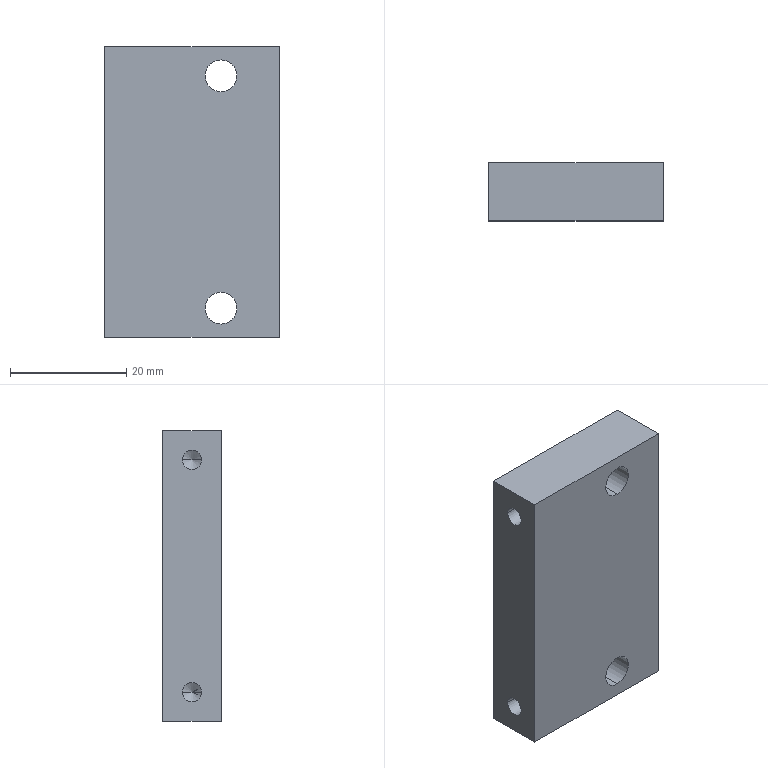Part | STEP file | 03-20 Lead screw head fixing plate 2 | 1 solid | 18 faces | box 30 x 10 x 50 mm | volume 14346 mm3 | cylinder 8 | plane 6 | cone 4 | commonest cylinder face diameters 3.3 x4 5.5 x4
STEP:
#1=CARTESIAN_POINT('',(0.,0.,0.));
#2=DIRECTION('',(0.,0.,1.));
#3=DIRECTION('',(1.,0.,0.));
#4=AXIS2_PLACEMENT_3D('',#1,#2,#3);
#5=CARTESIAN_POINT('',(20.,0.,22.75));
#6=VERTEX_POINT('',#5);
#7=CARTESIAN_POINT('',(20.,10.,22.75));
#8=VERTEX_POINT('',#7);
#9=CARTESIAN_POINT('',(20.,0.,22.75));
#10=DIRECTION('',(0.,1.,0.));
#11=VECTOR('',#10,1.);
#12=LINE('',#9,#11);
#13=CARTESIAN_POINT('',(20.,0.,20.));
#14=DIRECTION('',(0.,1.,0.));
#15=DIRECTION('',(0.,0.,1.));
#16=AXIS2_PLACEMENT_3D('',#13,#14,#15);
#17=CYLINDRICAL_SURFACE('',#16,2.75);
#18=CARTESIAN_POINT('',(6.283,0.));
#19=DIRECTION('',(0.,1.));
#20=VECTOR('',#19,1.);
#21=LINE('',#18,#20);
#22=(GEOMETRIC_REPRESENTATION_CONTEXT(2)PARAMETRIC_REPRESENTATION_CONTEXT()REPRESENTATION_CONTEXT('',''));
#23=DEFINITIONAL_REPRESENTATION('',(#21),#22);
#24=PCURVE('',#17,#23);
#25=CARTESIAN_POINT('',(20.,0.,20.));
#26=DIRECTION('',(0.,1.,0.));
#27=DIRECTION('',(0.,0.,1.));
#28=AXIS2_PLACEMENT_3D('',#25,#26,#27);
#29=CYLINDRICAL_SURFACE('',#28,2.75);
#30=CARTESIAN_POINT('',(0.,0.));
#31=DIRECTION('',(0.,1.));
#32=VECTOR('',#31,1.);
#33=LINE('',#30,#32);
#34=(GEOMETRIC_REPRESENTATION_CONTEXT(2)PARAMETRIC_REPRESENTATION_CONTEXT()REPRESENTATION_CONTEXT('',''));
#35=DEFINITIONAL_REPRESENTATION('',(#33),#34);
#36=PCURVE('',#29,#35);
#37=SURFACE_CURVE('',#12,(#24,#36),.PCURVE_S1.);
#38=EDGE_CURVE('',#6,#8,#37,.T.);
#39=ORIENTED_EDGE('',*,*,#38,.T.);
#40=CARTESIAN_POINT('',(20.,10.,17.25));
#41=VERTEX_POINT('',#40);
#42=CARTESIAN_POINT('',(20.,10.,20.));
#43=DIRECTION('',(0.,1.,0.));
#44=DIRECTION('',(0.,0.,1.));
#45=AXIS2_PLACEMENT_3D('',#42,#43,#44);
#46=CIRCLE('',#45,2.75);
#47=CARTESIAN_POINT('',(0.,10.));
#48=DIRECTION('',(1.,0.));
#49=VECTOR('',#48,1.);
#50=LINE('',#47,#49);
#51=(GEOMETRIC_REPRESENTATION_CONTEXT(2)PARAMETRIC_REPRESENTATION_CONTEXT()REPRESENTATION_CONTEXT('',''));
#52=DEFINITIONAL_REPRESENTATION('',(#50),#51);
#53=PCURVE('',#17,#52);
#54=CARTESIAN_POINT('',(0.,10.,25.));
#55=DIRECTION('',(0.,-1.,0.));
#56=DIRECTION('',(0.,0.,-1.));
#57=AXIS2_PLACEMENT_3D('',#54,#55,#56);
#58=PLANE('',#57);
#59=CARTESIAN_POINT('',(2.25,20.));
#60=CARTESIAN_POINT('',(2.25,24.763));
#61=CARTESIAN_POINT('',(6.375,22.382));
#62=CARTESIAN_POINT('',(10.5,20.));
#63=CARTESIAN_POINT('',(6.375,17.618));
#64=CARTESIAN_POINT('',(2.25,15.237));
#65=CARTESIAN_POINT('',(2.25,20.));
#66=(BOUNDED_CURVE()B_SPLINE_CURVE(2,(#59,#60,#61,#62,#63,#64,#65),.UNSPECIFIED.,.T.,.F.)B_SPLINE_CURVE_WITH_KNOTS((1,2,2,2,2,1),(-2.094,0.,2.094,4.189,6.283,8.378),.UNSPECIFIED.)CURVE()GEOMETRIC_REPRESENTATION_ITEM()RATIONAL_B_SPLINE_CURVE((1.,0.5,1.,0.5,1.,0.5,1.))REPRESENTATION_ITEM(''));
#67=(GEOMETRIC_REPRESENTATION_CONTEXT(2)PARAMETRIC_REPRESENTATION_CONTEXT()REPRESENTATION_CONTEXT('',''));
#68=DEFINITIONAL_REPRESENTATION('',(#66),#67);
#69=PCURVE('',#58,#68);
#70=SURFACE_CURVE('',#46,(#53,#69),.PCURVE_S1.);
#71=EDGE_CURVE('',#41,#8,#70,.T.);
#72=ORIENTED_EDGE('',*,*,#71,.F.);
#73=CARTESIAN_POINT('',(20.,0.,17.25));
#74=VERTEX_POINT('',#73);
#75=CARTESIAN_POINT('',(20.,0.,17.25));
#76=DIRECTION('',(0.,1.,0.));
#77=VECTOR('',#76,1.);
#78=LINE('',#75,#77);
#79=CARTESIAN_POINT('',(3.142,0.));
#80=DIRECTION('',(0.,1.));
#81=VECTOR('',#80,1.);
#82=LINE('',#79,#81);
#83=(GEOMETRIC_REPRESENTATION_CONTEXT(2)PARAMETRIC_REPRESENTATION_CONTEXT()REPRESENTATION_CONTEXT('',''));
#84=DEFINITIONAL_REPRESENTATION('',(#82),#83);
#85=PCURVE('',#17,#84);
#86=CARTESIAN_POINT('',(3.142,0.));
#87=DIRECTION('',(0.,1.));
#88=VECTOR('',#87,1.);
#89=LINE('',#86,#88);
#90=(GEOMETRIC_REPRESENTATION_CONTEXT(2)PARAMETRIC_REPRESENTATION_CONTEXT()REPRESENTATION_CONTEXT('',''));
#91=DEFINITIONAL_REPRESENTATION('',(#89),#90);
#92=PCURVE('',#29,#91);
#93=SURFACE_CURVE('',#78,(#85,#92),.PCURVE_S1.);
#94=EDGE_CURVE('',#74,#41,#93,.T.);
#95=ORIENTED_EDGE('',*,*,#94,.F.);
#96=CARTESIAN_POINT('',(20.,0.,20.));
#97=DIRECTION('',(0.,-1.,0.));
#98=DIRECTION('',(0.,0.,1.));
#99=AXIS2_PLACEMENT_3D('',#96,#97,#98);
#100=CIRCLE('',#99,2.75);
#101=CARTESIAN_POINT('',(6.283,0.));
#102=DIRECTION('',(-1.,0.));
#103=VECTOR('',#102,1.);
#104=LINE('',#101,#103);
#105=(GEOMETRIC_REPRESENTATION_CONTEXT(2)PARAMETRIC_REPRESENTATION_CONTEXT()REPRESENTATION_CONTEXT('',''));
#106=DEFINITIONAL_REPRESENTATION('',(#104),#105);
#107=PCURVE('',#17,#106);
#108=CARTESIAN_POINT('',(0.,0.,-25.));
#109=DIRECTION('',(0.,1.,0.));
#110=DIRECTION('',(0.,0.,1.));
#111=AXIS2_PLACEMENT_3D('',#108,#109,#110);
#112=PLANE('',#111);
#113=CARTESIAN_POINT('',(47.75,20.));
#114=CARTESIAN_POINT('',(47.75,15.237));
#115=CARTESIAN_POINT('',(43.625,17.618));
#116=CARTESIAN_POINT('',(39.5,20.));
#117=CARTESIAN_POINT('',(43.625,22.382));
#118=CARTESIAN_POINT('',(47.75,24.763));
#119=CARTESIAN_POINT('',(47.75,20.));
#120=(BOUNDED_CURVE()B_SPLINE_CURVE(2,(#113,#114,#115,#116,#117,#118,#119),.UNSPECIFIED.,.T.,.F.)B_SPLINE_CURVE_WITH_KNOTS((1,2,2,2,2,1),(-2.094,0.,2.094,4.189,6.283,8.378),.UNSPECIFIED.)CURVE()GEOMETRIC_REPRESENTATION_ITEM()RATIONAL_B_SPLINE_CURVE((1.,0.5,1.,0.5,1.,0.5,1.))REPRESENTATION_ITEM(''));
#121=(GEOMETRIC_REPRESENTATION_CONTEXT(2)PARAMETRIC_REPRESENTATION_CONTEXT()REPRESENTATION_CONTEXT('',''));
#122=DEFINITIONAL_REPRESENTATION('',(#120),#121);
#123=PCURVE('',#112,#122);
#124=SURFACE_CURVE('',#100,(#107,#123),.PCURVE_S1.);
#125=EDGE_CURVE('',#6,#74,#124,.T.);
#126=ORIENTED_EDGE('',*,*,#125,.F.);
#127=EDGE_LOOP('',(#39,#72,#95,#126));
#128=FACE_BOUND('',#127,.F.);
#129=ADVANCED_FACE('',(#128),#17,.F.);
#130=CARTESIAN_POINT('',(20.,0.,-17.25));
#131=VERTEX_POINT('',#130);
#132=CARTESIAN_POINT('',(20.,10.,-17.25));
#133=VERTEX_POINT('',#132);
#134=CARTESIAN_POINT('',(20.,0.,-17.25));
#135=DIRECTION('',(0.,1.,0.));
#136=VECTOR('',#135,1.);
#137=LINE('',#134,#136);
#138=CARTESIAN_POINT('',(20.,0.,-20.));
#139=DIRECTION('',(0.,1.,0.));
#140=DIRECTION('',(0.,0.,1.));
#141=AXIS2_PLACEMENT_3D('',#138,#139,#140);
#142=CYLINDRICAL_SURFACE('',#141,2.75);
#143=CARTESIAN_POINT('',(6.283,0.));
#144=DIRECTION('',(0.,1.));
#145=VECTOR('',#144,1.);
#146=LINE('',#143,#145);
#147=(GEOMETRIC_REPRESENTATION_CONTEXT(2)PARAMETRIC_REPRESENTATION_CONTEXT()REPRESENTATION_CONTEXT('',''));
#148=DEFINITIONAL_REPRESENTATION('',(#146),#147);
#149=PCURVE('',#142,#148);
#150=CARTESIAN_POINT('',(20.,0.,-20.));
#151=DIRECTION('',(0.,1.,0.));
#152=DIRECTION('',(0.,0.,1.));
#153=AXIS2_PLACEMENT_3D('',#150,#151,#152);
#154=CYLINDRICAL_SURFACE('',#153,2.75);
#155=CARTESIAN_POINT('',(0.,0.));
#156=DIRECTION('',(0.,1.));
#157=VECTOR('',#156,1.);
#158=LINE('',#155,#157);
#159=(GEOMETRIC_REPRESENTATION_CONTEXT(2)PARAMETRIC_REPRESENTATION_CONTEXT()REPRESENTATION_CONTEXT('',''));
#160=DEFINITIONAL_REPRESENTATION('',(#158),#159);
#161=PCURVE('',#154,#160);
#162=SURFACE_CURVE('',#137,(#149,#161),.PCURVE_S1.);
#163=EDGE_CURVE('',#131,#133,#162,.T.);
#164=ORIENTED_EDGE('',*,*,#163,.T.);
#165=CARTESIAN_POINT('',(20.,10.,-22.75));
#166=VERTEX_POINT('',#165);
#167=CARTESIAN_POINT('',(20.,10.,-20.));
#168=DIRECTION('',(0.,1.,0.));
#169=DIRECTION('',(0.,0.,1.));
#170=AXIS2_PLACEMENT_3D('',#167,#168,#169);
#171=CIRCLE('',#170,2.75);
#172=CARTESIAN_POINT('',(0.,10.));
#173=DIRECTION('',(1.,0.));
#174=VECTOR('',#173,1.);
#175=LINE('',#172,#174);
#176=(GEOMETRIC_REPRESENTATION_CONTEXT(2)PARAMETRIC_REPRESENTATION_CONTEXT()REPRESENTATION_CONTEXT('',''));
#177=DEFINITIONAL_REPRESENTATION('',(#175),#176);
#178=PCURVE('',#142,#177);
#179=CARTESIAN_POINT('',(42.25,20.));
#180=CARTESIAN_POINT('',(42.25,24.763));
#181=CARTESIAN_POINT('',(46.375,22.382));
#182=CARTESIAN_POINT('',(50.5,20.));
#183=CARTESIAN_POINT('',(46.375,17.618));
#184=CARTESIAN_POINT('',(42.25,15.237));
#185=CARTESIAN_POINT('',(42.25,20.));
#186=(BOUNDED_CURVE()B_SPLINE_CURVE(2,(#179,#180,#181,#182,#183,#184,#185),.UNSPECIFIED.,.T.,.F.)B_SPLINE_CURVE_WITH_KNOTS((1,2,2,2,2,1),(-2.094,0.,2.094,4.189,6.283,8.378),.UNSPECIFIED.)CURVE()GEOMETRIC_REPRESENTATION_ITEM()RATIONAL_B_SPLINE_CURVE((1.,0.5,1.,0.5,1.,0.5,1.))REPRESENTATION_ITEM(''));
#187=(GEOMETRIC_REPRESENTATION_CONTEXT(2)PARAMETRIC_REPRESENTATION_CONTEXT()REPRESENTATION_CONTEXT('',''));
#188=DEFINITIONAL_REPRESENTATION('',(#186),#187);
#189=PCURVE('',#58,#188);
#190=SURFACE_CURVE('',#171,(#178,#189),.PCURVE_S1.);
#191=EDGE_CURVE('',#166,#133,#190,.T.);
#192=ORIENTED_EDGE('',*,*,#191,.F.);
#193=CARTESIAN_POINT('',(20.,0.,-22.75));
#194=VERTEX_POINT('',#193);
#195=CARTESIAN_POINT('',(20.,0.,-22.75));
#196=DIRECTION('',(0.,1.,0.));
#197=VECTOR('',#196,1.);
#198=LINE('',#195,#197);
#199=CARTESIAN_POINT('',(3.142,0.));
#200=DIRECTION('',(0.,1.));
#201=VECTOR('',#200,1.);
#202=LINE('',#199,#201);
#203=(GEOMETRIC_REPRESENTATION_CONTEXT(2)PARAMETRIC_REPRESENTATION_CONTEXT()REPRESENTATION_CONTEXT('',''));
#204=DEFINITIONAL_REPRESENTATION('',(#202),#203);
#205=PCURVE('',#142,#204);
#206=CARTESIAN_POINT('',(3.142,0.));
#207=DIRECTION('',(0.,1.));
#208=VECTOR('',#207,1.);
#209=LINE('',#206,#208);
#210=(GEOMETRIC_REPRESENTATION_CONTEXT(2)PARAMETRIC_REPRESENTATION_CONTEXT()REPRESENTATION_CONTEXT('',''));
#211=DEFINITIONAL_REPRESENTATION('',(#209),#210);
#212=PCURVE('',#154,#211);
#213=SURFACE_CURVE('',#198,(#205,#212),.PCURVE_S1.);
#214=EDGE_CURVE('',#194,#166,#213,.T.);
#215=ORIENTED_EDGE('',*,*,#214,.F.);
#216=CARTESIAN_POINT('',(20.,0.,-20.));
#217=DIRECTION('',(0.,-1.,0.));
#218=DIRECTION('',(0.,0.,1.));
#219=AXIS2_PLACEMENT_3D('',#216,#217,#218);
#220=CIRCLE('',#219,2.75);
#221=CARTESIAN_POINT('',(6.283,0.));
#222=DIRECTION('',(-1.,0.));
#223=VECTOR('',#222,1.);
#224=LINE('',#221,#223);
#225=(GEOMETRIC_REPRESENTATION_CONTEXT(2)PARAMETRIC_REPRESENTATION_CONTEXT()REPRESENTATION_CONTEXT('',''));
#226=DEFINITIONAL_REPRESENTATION('',(#224),#225);
#227=PCURVE('',#142,#226);
#228=CARTESIAN_POINT('',(7.75,20.));
#229=CARTESIAN_POINT('',(7.75,15.237));
#230=CARTESIAN_POINT('',(3.625,17.618));
#231=CARTESIAN_POINT('',(-0.5,20.));
#232=CARTESIAN_POINT('',(3.625,22.382));
#233=CARTESIAN_POINT('',(7.75,24.763));
#234=CARTESIAN_POINT('',(7.75,20.));
#235=(BOUNDED_CURVE()B_SPLINE_CURVE(2,(#228,#229,#230,#231,#232,#233,#234),.UNSPECIFIED.,.T.,.F.)B_SPLINE_CURVE_WITH_KNOTS((1,2,2,2,2,1),(-2.094,0.,2.094,4.189,6.283,8.378),.UNSPECIFIED.)CURVE()GEOMETRIC_REPRESENTATION_ITEM()RATIONAL_B_SPLINE_CURVE((1.,0.5,1.,0.5,1.,0.5,1.))REPRESENTATION_ITEM(''));
#236=(GEOMETRIC_REPRESENTATION_CONTEXT(2)PARAMETRIC_REPRESENTATION_CONTEXT()REPRESENTATION_CONTEXT('',''));
#237=DEFINITIONAL_REPRESENTATION('',(#235),#236);
#238=PCURVE('',#112,#237);
#239=SURFACE_CURVE('',#220,(#227,#238),.PCURVE_S1.);
#240=EDGE_CURVE('',#131,#194,#239,.T.);
#241=ORIENTED_EDGE('',*,*,#240,.F.);
#242=EDGE_LOOP('',(#164,#192,#215,#241));
#243=FACE_BOUND('',#242,.F.);
#244=ADVANCED_FACE('',(#243),#142,.F.);
#245=CARTESIAN_POINT('',(10.1,3.35,20.));
#246=VERTEX_POINT('',#245);
#247=CARTESIAN_POINT('',(0.,3.35,20.));
#248=VERTEX_POINT('',#247);
#249=CARTESIAN_POINT('',(10.1,3.35,20.));
#250=DIRECTION('',(-1.,0.,0.));
#251=VECTOR('',#250,1.);
#252=LINE('',#249,#251);
#253=CARTESIAN_POINT('',(10.1,5.,20.));
#254=DIRECTION('',(-1.,0.,0.));
#255=DIRECTION('',(0.,-1.,0.));
#256=AXIS2_PLACEMENT_3D('',#253,#254,#255);
#257=CYLINDRICAL_SURFACE('',#256,1.65);
#258=CARTESIAN_POINT('',(6.283,0.));
#259=DIRECTION('',(0.,1.));
#260=VECTOR('',#259,1.);
#261=LINE('',#258,#260);
#262=(GEOMETRIC_REPRESENTATION_CONTEXT(2)PARAMETRIC_REPRESENTATION_CONTEXT()REPRESENTATION_CONTEXT('',''));
#263=DEFINITIONAL_REPRESENTATION('',(#261),#262);
#264=PCURVE('',#257,#263);
#265=CARTESIAN_POINT('',(10.1,5.,20.));
#266=DIRECTION('',(-1.,0.,0.));
#267=DIRECTION('',(0.,-1.,0.));
#268=AXIS2_PLACEMENT_3D('',#265,#266,#267);
#269=CYLINDRICAL_SURFACE('',#268,1.65);
#270=CARTESIAN_POINT('',(0.,0.));
#271=DIRECTION('',(0.,1.));
#272=VECTOR('',#271,1.);
#273=LINE('',#270,#272);
#274=(GEOMETRIC_REPRESENTATION_CONTEXT(2)PARAMETRIC_REPRESENTATION_CONTEXT()REPRESENTATION_CONTEXT('',''));
#275=DEFINITIONAL_REPRESENTATION('',(#273),#274);
#276=PCURVE('',#269,#275);
#277=SURFACE_CURVE('',#252,(#264,#276),.PCURVE_S1.);
#278=EDGE_CURVE('',#246,#248,#277,.T.);
#279=ORIENTED_EDGE('',*,*,#278,.T.);
#280=CARTESIAN_POINT('',(0.,6.65,20.));
#281=VERTEX_POINT('',#280);
#282=CARTESIAN_POINT('',(0.,5.,20.));
#283=DIRECTION('',(1.,0.,0.));
#284=DIRECTION('',(0.,-1.,0.));
#285=AXIS2_PLACEMENT_3D('',#282,#283,#284);
#286=CIRCLE('',#285,1.65);
#287=CARTESIAN_POINT('',(6.283,10.1));
#288=DIRECTION('',(-1.,0.));
#289=VECTOR('',#288,1.);
#290=LINE('',#287,#289);
#291=(GEOMETRIC_REPRESENTATION_CONTEXT(2)PARAMETRIC_REPRESENTATION_CONTEXT()REPRESENTATION_CONTEXT('',''));
#292=DEFINITIONAL_REPRESENTATION('',(#290),#291);
#293=PCURVE('',#257,#292);
#294=CARTESIAN_POINT('',(0.,0.,-25.));
#295=DIRECTION('',(-1.,0.,0.));
#296=DIRECTION('',(0.,0.,1.));
#297=AXIS2_PLACEMENT_3D('',#294,#295,#296);
#298=PLANE('',#297);
#299=CARTESIAN_POINT('',(45.,3.35));
#300=CARTESIAN_POINT('',(42.142,3.35));
#301=CARTESIAN_POINT('',(43.571,5.825));
#302=CARTESIAN_POINT('',(45.,8.3));
#303=CARTESIAN_POINT('',(46.429,5.825));
#304=CARTESIAN_POINT('',(47.858,3.35));
#305=CARTESIAN_POINT('',(45.,3.35));
#306=(BOUNDED_CURVE()B_SPLINE_CURVE(2,(#299,#300,#301,#302,#303,#304,#305),.UNSPECIFIED.,.T.,.F.)B_SPLINE_CURVE_WITH_KNOTS((1,2,2,2,2,1),(-2.094,0.,2.094,4.189,6.283,8.378),.UNSPECIFIED.)CURVE()GEOMETRIC_REPRESENTATION_ITEM()RATIONAL_B_SPLINE_CURVE((1.,0.5,1.,0.5,1.,0.5,1.))REPRESENTATION_ITEM(''));
#307=(GEOMETRIC_REPRESENTATION_CONTEXT(2)PARAMETRIC_REPRESENTATION_CONTEXT()REPRESENTATION_CONTEXT('',''));
#308=DEFINITIONAL_REPRESENTATION('',(#306),#307);
#309=PCURVE('',#298,#308);
#310=SURFACE_CURVE('',#286,(#293,#309),.PCURVE_S1.);
#311=EDGE_CURVE('',#248,#281,#310,.T.);
#312=ORIENTED_EDGE('',*,*,#311,.T.);
#313=CARTESIAN_POINT('',(10.1,6.65,20.));
#314=VERTEX_POINT('',#313);
#315=CARTESIAN_POINT('',(10.1,6.65,20.));
#316=DIRECTION('',(-1.,0.,0.));
#317=VECTOR('',#316,1.);
#318=LINE('',#315,#317);
#319=CARTESIAN_POINT('',(3.142,0.));
#320=DIRECTION('',(0.,1.));
#321=VECTOR('',#320,1.);
#322=LINE('',#319,#321);
#323=(GEOMETRIC_REPRESENTATION_CONTEXT(2)PARAMETRIC_REPRESENTATION_CONTEXT()REPRESENTATION_CONTEXT('',''));
#324=DEFINITIONAL_REPRESENTATION('',(#322),#323);
#325=PCURVE('',#257,#324);
#326=CARTESIAN_POINT('',(3.142,0.));
#327=DIRECTION('',(0.,1.));
#328=VECTOR('',#327,1.);
#329=LINE('',#326,#328);
#330=(GEOMETRIC_REPRESENTATION_CONTEXT(2)PARAMETRIC_REPRESENTATION_CONTEXT()REPRESENTATION_CONTEXT('',''));
#331=DEFINITIONAL_REPRESENTATION('',(#329),#330);
#332=PCURVE('',#269,#331);
#333=SURFACE_CURVE('',#318,(#325,#332),.PCURVE_S1.);
#334=EDGE_CURVE('',#314,#281,#333,.T.);
#335=ORIENTED_EDGE('',*,*,#334,.F.);
#336=CARTESIAN_POINT('',(10.1,5.,20.));
#337=DIRECTION('',(1.,0.,0.));
#338=DIRECTION('',(0.,0.,1.));
#339=AXIS2_PLACEMENT_3D('',#336,#337,#338);
#340=CIRCLE('',#339,1.65);
#341=CARTESIAN_POINT('',(7.854,0.));
#342=DIRECTION('',(-1.,0.));
#343=VECTOR('',#342,1.);
#344=LINE('',#341,#343);
#345=(GEOMETRIC_REPRESENTATION_CONTEXT(2)PARAMETRIC_REPRESENTATION_CONTEXT()REPRESENTATION_CONTEXT('',''));
#346=DEFINITIONAL_REPRESENTATION('',(#344),#345);
#347=PCURVE('',#257,#346);
#348=CARTESIAN_POINT('',(-988.909,5.,20.));
#349=DIRECTION('',(-1.,0.,0.));
#350=DIRECTION('',(0.,-1.,0.));
#351=AXIS2_PLACEMENT_3D('',#348,#349,#350);
#352=CONICAL_SURFACE('',#351,1664.279,1.03);
#353=CARTESIAN_POINT('',(7.854,-999.009));
#354=DIRECTION('',(-1.,0.));
#355=VECTOR('',#354,1.);
#356=LINE('',#353,#355);
#357=(GEOMETRIC_REPRESENTATION_CONTEXT(2)PARAMETRIC_REPRESENTATION_CONTEXT()REPRESENTATION_CONTEXT('',''));
#358=DEFINITIONAL_REPRESENTATION('',(#356),#357);
#359=PCURVE('',#352,#358);
#360=SURFACE_CURVE('',#340,(#347,#359),.PCURVE_S1.);
#361=EDGE_CURVE('',#246,#314,#360,.T.);
#362=ORIENTED_EDGE('',*,*,#361,.F.);
#363=EDGE_LOOP('',(#279,#312,#335,#362));
#364=FACE_BOUND('',#363,.F.);
#365=ADVANCED_FACE('',(#364),#257,.F.);
#366=CARTESIAN_POINT('',(10.1,3.35,-20.));
#367=VERTEX_POINT('',#366);
#368=CARTESIAN_POINT('',(0.,3.35,-20.));
#369=VERTEX_POINT('',#368);
#370=CARTESIAN_POINT('',(10.1,3.35,-20.));
#371=DIRECTION('',(-1.,0.,0.));
#372=VECTOR('',#371,1.);
#373=LINE('',#370,#372);
#374=CARTESIAN_POINT('',(10.1,5.,-20.));
#375=DIRECTION('',(-1.,0.,0.));
#376=DIRECTION('',(0.,-1.,0.));
#377=AXIS2_PLACEMENT_3D('',#374,#375,#376);
#378=CYLINDRICAL_SURFACE('',#377,1.65);
#379=CARTESIAN_POINT('',(6.283,0.));
#380=DIRECTION('',(0.,1.));
#381=VECTOR('',#380,1.);
#382=LINE('',#379,#381);
#383=(GEOMETRIC_REPRESENTATION_CONTEXT(2)PARAMETRIC_REPRESENTATION_CONTEXT()REPRESENTATION_CONTEXT('',''));
#384=DEFINITIONAL_REPRESENTATION('',(#382),#383);
#385=PCURVE('',#378,#384);
#386=CARTESIAN_POINT('',(10.1,5.,-20.));
#387=DIRECTION('',(-1.,0.,0.));
#388=DIRECTION('',(0.,-1.,0.));
#389=AXIS2_PLACEMENT_3D('',#386,#387,#388);
#390=CYLINDRICAL_SURFACE('',#389,1.65);
#391=CARTESIAN_POINT('',(0.,0.));
#392=DIRECTION('',(0.,1.));
#393=VECTOR('',#392,1.);
#394=LINE('',#391,#393);
#395=(GEOMETRIC_REPRESENTATION_CONTEXT(2)PARAMETRIC_REPRESENTATION_CONTEXT()REPRESENTATION_CONTEXT('',''));
#396=DEFINITIONAL_REPRESENTATION('',(#394),#395);
#397=PCURVE('',#390,#396);
#398=SURFACE_CURVE('',#373,(#385,#397),.PCURVE_S1.);
#399=EDGE_CURVE('',#367,#369,#398,.T.);
#400=ORIENTED_EDGE('',*,*,#399,.T.);
#401=CARTESIAN_POINT('',(0.,6.65,-20.));
#402=VERTEX_POINT('',#401);
#403=CARTESIAN_POINT('',(0.,5.,-20.));
#404=DIRECTION('',(1.,0.,0.));
#405=DIRECTION('',(0.,-1.,0.));
#406=AXIS2_PLACEMENT_3D('',#403,#404,#405);
#407=CIRCLE('',#406,1.65);
#408=CARTESIAN_POINT('',(6.283,10.1));
#409=DIRECTION('',(-1.,0.));
#410=VECTOR('',#409,1.);
#411=LINE('',#408,#410);
#412=(GEOMETRIC_REPRESENTATION_CONTEXT(2)PARAMETRIC_REPRESENTATION_CONTEXT()REPRESENTATION_CONTEXT('',''));
#413=DEFINITIONAL_REPRESENTATION('',(#411),#412);
#414=PCURVE('',#378,#413);
#415=CARTESIAN_POINT('',(5.,3.35));
#416=CARTESIAN_POINT('',(2.142,3.35));
#417=CARTESIAN_POINT('',(3.571,5.825));
#418=CARTESIAN_POINT('',(5.,8.3));
#419=CARTESIAN_POINT('',(6.429,5.825));
#420=CARTESIAN_POINT('',(7.858,3.35));
#421=CARTESIAN_POINT('',(5.,3.35));
#422=(BOUNDED_CURVE()B_SPLINE_CURVE(2,(#415,#416,#417,#418,#419,#420,#421),.UNSPECIFIED.,.T.,.F.)B_SPLINE_CURVE_WITH_KNOTS((1,2,2,2,2,1),(-2.094,0.,2.094,4.189,6.283,8.378),.UNSPECIFIED.)CURVE()GEOMETRIC_REPRESENTATION_ITEM()RATIONAL_B_SPLINE_CURVE((1.,0.5,1.,0.5,1.,0.5,1.))REPRESENTATION_ITEM(''));
#423=(GEOMETRIC_REPRESENTATION_CONTEXT(2)PARAMETRIC_REPRESENTATION_CONTEXT()REPRESENTATION_CONTEXT('',''));
#424=DEFINITIONAL_REPRESENTATION('',(#422),#423);
#425=PCURVE('',#298,#424);
#426=SURFACE_CURVE('',#407,(#414,#425),.PCURVE_S1.);
#427=EDGE_CURVE('',#369,#402,#426,.T.);
#428=ORIENTED_EDGE('',*,*,#427,.T.);
#429=CARTESIAN_POINT('',(10.1,6.65,-20.));
#430=VERTEX_POINT('',#429);
#431=CARTESIAN_POINT('',(10.1,6.65,-20.));
#432=DIRECTION('',(-1.,0.,0.));
#433=VECTOR('',#432,1.);
#434=LINE('',#431,#433);
#435=CARTESIAN_POINT('',(3.142,0.));
#436=DIRECTION('',(0.,1.));
#437=VECTOR('',#436,1.);
#438=LINE('',#435,#437);
#439=(GEOMETRIC_REPRESENTATION_CONTEXT(2)PARAMETRIC_REPRESENTATION_CONTEXT()REPRESENTATION_CONTEXT('',''));
#440=DEFINITIONAL_REPRESENTATION('',(#438),#439);
#441=PCURVE('',#378,#440);
#442=CARTESIAN_POINT('',(3.142,0.));
#443=DIRECTION('',(0.,1.));
#444=VECTOR('',#443,1.);
#445=LINE('',#442,#444);
#446=(GEOMETRIC_REPRESENTATION_CONTEXT(2)PARAMETRIC_REPRESENTATION_CONTEXT()REPRESENTATION_CONTEXT('',''));
#447=DEFINITIONAL_REPRESENTATION('',(#445),#446);
#448=PCURVE('',#390,#447);
#449=SURFACE_CURVE('',#434,(#441,#448),.PCURVE_S1.);
#450=EDGE_CURVE('',#430,#402,#449,.T.);
#451=ORIENTED_EDGE('',*,*,#450,.F.);
#452=CARTESIAN_POINT('',(10.1,5.,-20.));
#453=DIRECTION('',(1.,0.,0.));
#454=DIRECTION('',(0.,0.,1.));
#455=AXIS2_PLACEMENT_3D('',#452,#453,#454);
#456=CIRCLE('',#455,1.65);
#457=CARTESIAN_POINT('',(7.854,0.));
#458=DIRECTION('',(-1.,0.));
#459=VECTOR('',#458,1.);
#460=LINE('',#457,#459);
#461=(GEOMETRIC_REPRESENTATION_CONTEXT(2)PARAMETRIC_REPRESENTATION_CONTEXT()REPRESENTATION_CONTEXT('',''));
#462=DEFINITIONAL_REPRESENTATION('',(#460),#461);
#463=PCURVE('',#378,#462);
#464=CARTESIAN_POINT('',(-988.909,5.,-20.));
#465=DIRECTION('',(-1.,0.,0.));
#466=DIRECTION('',(0.,-1.,0.));
#467=AXIS2_PLACEMENT_3D('',#464,#465,#466);
#468=CONICAL_SURFACE('',#467,1664.279,1.03);
#469=CARTESIAN_POINT('',(7.854,-999.009));
#470=DIRECTION('',(-1.,0.));
#471=VECTOR('',#470,1.);
#472=LINE('',#469,#471);
#473=(GEOMETRIC_REPRESENTATION_CONTEXT(2)PARAMETRIC_REPRESENTATION_CONTEXT()REPRESENTATION_CONTEXT('',''));
#474=DEFINITIONAL_REPRESENTATION('',(#472),#473);
#475=PCURVE('',#468,#474);
#476=SURFACE_CURVE('',#456,(#463,#475),.PCURVE_S1.);
#477=EDGE_CURVE('',#367,#430,#476,.T.);
#478=ORIENTED_EDGE('',*,*,#477,.F.);
#479=EDGE_LOOP('',(#400,#428,#451,#478));
#480=FACE_BOUND('',#479,.F.);
#481=ADVANCED_FACE('',(#480),#378,.F.);
#482=ORIENTED_EDGE('',*,*,#361,.T.);
#483=CARTESIAN_POINT('',(11.091,5.,20.));
#484=VERTEX_POINT('',#483);
#485=CARTESIAN_POINT('',(11.091,5.,20.));
#486=DIRECTION('',(-0.515,0.8572,0.));
#487=VECTOR('',#486,1.);
#488=LINE('',#485,#487);
#489=CARTESIAN_POINT('',(3.142,-1000.));
#490=CARTESIAN_POINT('',(3.142,-999.985));
#491=CARTESIAN_POINT('',(3.142,-999.955));
#492=CARTESIAN_POINT('',(3.142,-999.91));
#493=CARTESIAN_POINT('',(3.142,-999.865));
#494=CARTESIAN_POINT('',(3.142,-999.82));
#495=CARTESIAN_POINT('',(3.142,-999.775));
#496=CARTESIAN_POINT('',(3.142,-999.73));
#497=CARTESIAN_POINT('',(3.142,-999.685));
#498=CARTESIAN_POINT('',(3.142,-999.639));
#499=CARTESIAN_POINT('',(3.142,-999.594));
#500=CARTESIAN_POINT('',(3.142,-999.549));
#501=CARTESIAN_POINT('',(3.142,-999.504));
#502=CARTESIAN_POINT('',(3.142,-999.459));
#503=CARTESIAN_POINT('',(3.142,-999.414));
#504=CARTESIAN_POINT('',(3.142,-999.369));
#505=CARTESIAN_POINT('',(3.142,-999.324));
#506=CARTESIAN_POINT('',(3.142,-999.279));
#507=CARTESIAN_POINT('',(3.142,-999.234));
#508=CARTESIAN_POINT('',(3.142,-999.189));
#509=CARTESIAN_POINT('',(3.142,-999.144));
#510=CARTESIAN_POINT('',(3.142,-999.099));
#511=CARTESIAN_POINT('',(3.142,-999.054));
#512=CARTESIAN_POINT('',(3.142,-999.024));
#513=CARTESIAN_POINT('',(3.142,-999.009));
#514=B_SPLINE_CURVE_WITH_KNOTS('',3,(#489,#490,#491,#492,#493,#494,#495,#496,#497,#498,#499,#500,#501,#502,#503,#504,#505,#506,#507,#508,#509,#510,#511,#512,#513),.UNSPECIFIED.,.F.,.F.,(4,1,1,1,1,1,1,1,1,1,1,1,1,1,1,1,1,1,1,1,1,1,4),(0.,0.0875,0.175,0.2625,0.35,0.4375,0.525,0.6125,0.7,0.7875,0.875,0.9625,1.05,1.137,1.225,1.312,1.4,1.487,1.575,1.662,1.75,1.837,1.925),.UNSPECIFIED.);
#515=(GEOMETRIC_REPRESENTATION_CONTEXT(2)PARAMETRIC_REPRESENTATION_CONTEXT()REPRESENTATION_CONTEXT('',''));
#516=DEFINITIONAL_REPRESENTATION('',(#514),#515);
#517=PCURVE('',#352,#516);
#518=CARTESIAN_POINT('',(-988.909,5.,20.));
#519=DIRECTION('',(-1.,0.,0.));
#520=DIRECTION('',(0.,-1.,0.));
#521=AXIS2_PLACEMENT_3D('',#518,#519,#520);
#522=CONICAL_SURFACE('',#521,1664.279,1.03);
#523=CARTESIAN_POINT('',(3.142,-1000.));
#524=CARTESIAN_POINT('',(3.142,-999.985));
#525=CARTESIAN_POINT('',(3.142,-999.955));
#526=CARTESIAN_POINT('',(3.142,-999.91));
#527=CARTESIAN_POINT('',(3.142,-999.865));
#528=CARTESIAN_POINT('',(3.142,-999.82));
#529=CARTESIAN_POINT('',(3.142,-999.775));
#530=CARTESIAN_POINT('',(3.142,-999.73));
#531=CARTESIAN_POINT('',(3.142,-999.685));
#532=CARTESIAN_POINT('',(3.142,-999.639));
#533=CARTESIAN_POINT('',(3.142,-999.594));
#534=CARTESIAN_POINT('',(3.142,-999.549));
#535=CARTESIAN_POINT('',(3.142,-999.504));
#536=CARTESIAN_POINT('',(3.142,-999.459));
#537=CARTESIAN_POINT('',(3.142,-999.414));
#538=CARTESIAN_POINT('',(3.142,-999.369));
#539=CARTESIAN_POINT('',(3.142,-999.324));
#540=CARTESIAN_POINT('',(3.142,-999.279));
#541=CARTESIAN_POINT('',(3.142,-999.234));
#542=CARTESIAN_POINT('',(3.142,-999.189));
#543=CARTESIAN_POINT('',(3.142,-999.144));
#544=CARTESIAN_POINT('',(3.142,-999.099));
#545=CARTESIAN_POINT('',(3.142,-999.054));
#546=CARTESIAN_POINT('',(3.142,-999.024));
#547=CARTESIAN_POINT('',(3.142,-999.009));
#548=B_SPLINE_CURVE_WITH_KNOTS('',3,(#523,#524,#525,#526,#527,#528,#529,#530,#531,#532,#533,#534,#535,#536,#537,#538,#539,#540,#541,#542,#543,#544,#545,#546,#547),.UNSPECIFIED.,.F.,.F.,(4,1,1,1,1,1,1,1,1,1,1,1,1,1,1,1,1,1,1,1,1,1,4),(0.,0.0875,0.175,0.2625,0.35,0.4375,0.525,0.6125,0.7,0.7875,0.875,0.9625,1.05,1.137,1.225,1.312,1.4,1.487,1.575,1.662,1.75,1.837,1.925),.UNSPECIFIED.);
#549=(GEOMETRIC_REPRESENTATION_CONTEXT(2)PARAMETRIC_REPRESENTATION_CONTEXT()REPRESENTATION_CONTEXT('',''));
#550=DEFINITIONAL_REPRESENTATION('',(#548),#549);
#551=PCURVE('',#522,#550);
#552=SURFACE_CURVE('',#488,(#517,#551),.PCURVE_S1.);
#553=EDGE_CURVE('',#484,#314,#552,.T.);
#554=ORIENTED_EDGE('',*,*,#553,.F.);
#555=CARTESIAN_POINT('',(11.091,5.,20.));
#556=DIRECTION('',(-0.515,-0.8572,0.));
#557=VECTOR('',#556,1.);
#558=LINE('',#555,#557);
#559=CARTESIAN_POINT('',(6.283,-1000.));
#560=CARTESIAN_POINT('',(6.283,-999.985));
#561=CARTESIAN_POINT('',(6.283,-999.955));
#562=CARTESIAN_POINT('',(6.283,-999.91));
#563=CARTESIAN_POINT('',(6.283,-999.865));
#564=CARTESIAN_POINT('',(6.283,-999.82));
#565=CARTESIAN_POINT('',(6.283,-999.775));
#566=CARTESIAN_POINT('',(6.283,-999.73));
#567=CARTESIAN_POINT('',(6.283,-999.685));
#568=CARTESIAN_POINT('',(6.283,-999.639));
#569=CARTESIAN_POINT('',(6.283,-999.594));
#570=CARTESIAN_POINT('',(6.283,-999.549));
#571=CARTESIAN_POINT('',(6.283,-999.504));
#572=CARTESIAN_POINT('',(6.283,-999.459));
#573=CARTESIAN_POINT('',(6.283,-999.414));
#574=CARTESIAN_POINT('',(6.283,-999.369));
#575=CARTESIAN_POINT('',(6.283,-999.324));
#576=CARTESIAN_POINT('',(6.283,-999.279));
#577=CARTESIAN_POINT('',(6.283,-999.234));
#578=CARTESIAN_POINT('',(6.283,-999.189));
#579=CARTESIAN_POINT('',(6.283,-999.144));
#580=CARTESIAN_POINT('',(6.283,-999.099));
#581=CARTESIAN_POINT('',(6.283,-999.054));
#582=CARTESIAN_POINT('',(6.283,-999.024));
#583=CARTESIAN_POINT('',(6.283,-999.009));
#584=B_SPLINE_CURVE_WITH_KNOTS('',3,(#559,#560,#561,#562,#563,#564,#565,#566,#567,#568,#569,#570,#571,#572,#573,#574,#575,#576,#577,#578,#579,#580,#581,#582,#583),.UNSPECIFIED.,.F.,.F.,(4,1,1,1,1,1,1,1,1,1,1,1,1,1,1,1,1,1,1,1,1,1,4),(0.,0.0875,0.175,0.2625,0.35,0.4375,0.525,0.6125,0.7,0.7875,0.875,0.9625,1.05,1.137,1.225,1.312,1.4,1.487,1.575,1.662,1.75,1.837,1.925),.UNSPECIFIED.);
#585=(GEOMETRIC_REPRESENTATION_CONTEXT(2)PARAMETRIC_REPRESENTATION_CONTEXT()REPRESENTATION_CONTEXT('',''));
#586=DEFINITIONAL_REPRESENTATION('',(#584),#585);
#587=PCURVE('',#352,#586);
#588=CARTESIAN_POINT('',(0.,-1000.));
#589=CARTESIAN_POINT('',(0.,-999.985));
#590=CARTESIAN_POINT('',(0.,-999.955));
#591=CARTESIAN_POINT('',(0.,-999.91));
#592=CARTESIAN_POINT('',(0.,-999.865));
#593=CARTESIAN_POINT('',(0.,-999.82));
#594=CARTESIAN_POINT('',(0.,-999.775));
#595=CARTESIAN_POINT('',(0.,-999.73));
#596=CARTESIAN_POINT('',(0.,-999.685));
#597=CARTESIAN_POINT('',(0.,-999.639));
#598=CARTESIAN_POINT('',(0.,-999.594));
#599=CARTESIAN_POINT('',(0.,-999.549));
#600=CARTESIAN_POINT('',(0.,-999.504));
#601=CARTESIAN_POINT('',(0.,-999.459));
#602=CARTESIAN_POINT('',(0.,-999.414));
#603=CARTESIAN_POINT('',(0.,-999.369));
#604=CARTESIAN_POINT('',(0.,-999.324));
#605=CARTESIAN_POINT('',(0.,-999.279));
#606=CARTESIAN_POINT('',(0.,-999.234));
#607=CARTESIAN_POINT('',(0.,-999.189));
#608=CARTESIAN_POINT('',(0.,-999.144));
#609=CARTESIAN_POINT('',(0.,-999.099));
#610=CARTESIAN_POINT('',(0.,-999.054));
#611=CARTESIAN_POINT('',(0.,-999.024));
#612=CARTESIAN_POINT('',(0.,-999.009));
#613=B_SPLINE_CURVE_WITH_KNOTS('',3,(#588,#589,#590,#591,#592,#593,#594,#595,#596,#597,#598,#599,#600,#601,#602,#603,#604,#605,#606,#607,#608,#609,#610,#611,#612),.UNSPECIFIED.,.F.,.F.,(4,1,1,1,1,1,1,1,1,1,1,1,1,1,1,1,1,1,1,1,1,1,4),(0.,0.0875,0.175,0.2625,0.35,0.4375,0.525,0.6125,0.7,0.7875,0.875,0.9625,1.05,1.137,1.225,1.312,1.4,1.487,1.575,1.662,1.75,1.837,1.925),.UNSPECIFIED.);
#614=(GEOMETRIC_REPRESENTATION_CONTEXT(2)PARAMETRIC_REPRESENTATION_CONTEXT()REPRESENTATION_CONTEXT('',''));
#615=DEFINITIONAL_REPRESENTATION('',(#613),#614);
#616=PCURVE('',#522,#615);
#617=SURFACE_CURVE('',#558,(#587,#616),.PCURVE_S1.);
#618=EDGE_CURVE('',#484,#246,#617,.T.);
#619=ORIENTED_EDGE('',*,*,#618,.T.);
#620=EDGE_LOOP('',(#482,#554,#619));
#621=FACE_BOUND('',#620,.F.);
#622=ADVANCED_FACE('',(#621),#352,.F.);
#623=ORIENTED_EDGE('',*,*,#477,.T.);
#624=CARTESIAN_POINT('',(11.091,5.,-20.));
#625=VERTEX_POINT('',#624);
#626=CARTESIAN_POINT('',(11.091,5.,-20.));
#627=DIRECTION('',(-0.515,0.8572,0.));
#628=VECTOR('',#627,1.);
#629=LINE('',#626,#628);
#630=CARTESIAN_POINT('',(3.142,-1000.));
#631=CARTESIAN_POINT('',(3.142,-999.985));
#632=CARTESIAN_POINT('',(3.142,-999.955));
#633=CARTESIAN_POINT('',(3.142,-999.91));
#634=CARTESIAN_POINT('',(3.142,-999.865));
#635=CARTESIAN_POINT('',(3.142,-999.82));
#636=CARTESIAN_POINT('',(3.142,-999.775));
#637=CARTESIAN_POINT('',(3.142,-999.73));
#638=CARTESIAN_POINT('',(3.142,-999.685));
#639=CARTESIAN_POINT('',(3.142,-999.639));
#640=CARTESIAN_POINT('',(3.142,-999.594));
#641=CARTESIAN_POINT('',(3.142,-999.549));
#642=CARTESIAN_POINT('',(3.142,-999.504));
#643=CARTESIAN_POINT('',(3.142,-999.459));
#644=CARTESIAN_POINT('',(3.142,-999.414));
#645=CARTESIAN_POINT('',(3.142,-999.369));
#646=CARTESIAN_POINT('',(3.142,-999.324));
#647=CARTESIAN_POINT('',(3.142,-999.279));
#648=CARTESIAN_POINT('',(3.142,-999.234));
#649=CARTESIAN_POINT('',(3.142,-999.189));
#650=CARTESIAN_POINT('',(3.142,-999.144));
#651=CARTESIAN_POINT('',(3.142,-999.099));
#652=CARTESIAN_POINT('',(3.142,-999.054));
#653=CARTESIAN_POINT('',(3.142,-999.024));
#654=CARTESIAN_POINT('',(3.142,-999.009));
#655=B_SPLINE_CURVE_WITH_KNOTS('',3,(#630,#631,#632,#633,#634,#635,#636,#637,#638,#639,#640,#641,#642,#643,#644,#645,#646,#647,#648,#649,#650,#651,#652,#653,#654),.UNSPECIFIED.,.F.,.F.,(4,1,1,1,1,1,1,1,1,1,1,1,1,1,1,1,1,1,1,1,1,1,4),(0.,0.0875,0.175,0.2625,0.35,0.4375,0.525,0.6125,0.7,0.7875,0.875,0.9625,1.05,1.137,1.225,1.312,1.4,1.487,1.575,1.662,1.75,1.837,1.925),.QUASI_UNIFORM_KNOTS.);
#656=(GEOMETRIC_REPRESENTATION_CONTEXT(2)PARAMETRIC_REPRESENTATION_CONTEXT()REPRESENTATION_CONTEXT('',''));
#657=DEFINITIONAL_REPRESENTATION('',(#655),#656);
#658=PCURVE('',#468,#657);
#659=CARTESIAN_POINT('',(-988.909,5.,-20.));
#660=DIRECTION('',(-1.,0.,0.));
#661=DIRECTION('',(0.,-1.,0.));
#662=AXIS2_PLACEMENT_3D('',#659,#660,#661);
#663=CONICAL_SURFACE('',#662,1664.279,1.03);
#664=CARTESIAN_POINT('',(3.142,-1000.));
#665=CARTESIAN_POINT('',(3.142,-999.985));
#666=CARTESIAN_POINT('',(3.142,-999.955));
#667=CARTESIAN_POINT('',(3.142,-999.91));
#668=CARTESIAN_POINT('',(3.142,-999.865));
#669=CARTESIAN_POINT('',(3.142,-999.82));
#670=CARTESIAN_POINT('',(3.142,-999.775));
#671=CARTESIAN_POINT('',(3.142,-999.73));
#672=CARTESIAN_POINT('',(3.142,-999.685));
#673=CARTESIAN_POINT('',(3.142,-999.639));
#674=CARTESIAN_POINT('',(3.142,-999.594));
#675=CARTESIAN_POINT('',(3.142,-999.549));
#676=CARTESIAN_POINT('',(3.142,-999.504));
#677=CARTESIAN_POINT('',(3.142,-999.459));
#678=CARTESIAN_POINT('',(3.142,-999.414));
#679=CARTESIAN_POINT('',(3.142,-999.369));
#680=CARTESIAN_POINT('',(3.142,-999.324));
#681=CARTESIAN_POINT('',(3.142,-999.279));
#682=CARTESIAN_POINT('',(3.142,-999.234));
#683=CARTESIAN_POINT('',(3.142,-999.189));
#684=CARTESIAN_POINT('',(3.142,-999.144));
#685=CARTESIAN_POINT('',(3.142,-999.099));
#686=CARTESIAN_POINT('',(3.142,-999.054));
#687=CARTESIAN_POINT('',(3.142,-999.024));
#688=CARTESIAN_POINT('',(3.142,-999.009));
#689=B_SPLINE_CURVE_WITH_KNOTS('',3,(#664,#665,#666,#667,#668,#669,#670,#671,#672,#673,#674,#675,#676,#677,#678,#679,#680,#681,#682,#683,#684,#685,#686,#687,#688),.UNSPECIFIED.,.F.,.F.,(4,1,1,1,1,1,1,1,1,1,1,1,1,1,1,1,1,1,1,1,1,1,4),(0.,0.0875,0.175,0.2625,0.35,0.4375,0.525,0.6125,0.7,0.7875,0.875,0.9625,1.05,1.137,1.225,1.312,1.4,1.487,1.575,1.662,1.75,1.837,1.925),.QUASI_UNIFORM_KNOTS.);
#690=(GEOMETRIC_REPRESENTATION_CONTEXT(2)PARAMETRIC_REPRESENTATION_CONTEXT()REPRESENTATION_CONTEXT('',''));
#691=DEFINITIONAL_REPRESENTATION('',(#689),#690);
#692=PCURVE('',#663,#691);
#693=SURFACE_CURVE('',#629,(#658,#692),.PCURVE_S1.);
#694=EDGE_CURVE('',#625,#430,#693,.T.);
#695=ORIENTED_EDGE('',*,*,#694,.F.);
#696=CARTESIAN_POINT('',(11.091,5.,-20.));
#697=DIRECTION('',(-0.515,-0.8572,0.));
#698=VECTOR('',#697,1.);
#699=LINE('',#696,#698);
#700=CARTESIAN_POINT('',(6.283,-1000.));
#701=DIRECTION('',(0.,1.));
#702=VECTOR('',#701,1.);
#703=LINE('',#700,#702);
#704=(GEOMETRIC_REPRESENTATION_CONTEXT(2)PARAMETRIC_REPRESENTATION_CONTEXT()REPRESENTATION_CONTEXT('',''));
#705=DEFINITIONAL_REPRESENTATION('',(#703),#704);
#706=PCURVE('',#468,#705);
#707=CARTESIAN_POINT('',(0.,-1000.));
#708=DIRECTION('',(0.,1.));
#709=VECTOR('',#708,1.);
#710=LINE('',#707,#709);
#711=(GEOMETRIC_REPRESENTATION_CONTEXT(2)PARAMETRIC_REPRESENTATION_CONTEXT()REPRESENTATION_CONTEXT('',''));
#712=DEFINITIONAL_REPRESENTATION('',(#710),#711);
#713=PCURVE('',#663,#712);
#714=SURFACE_CURVE('',#699,(#706,#713),.PCURVE_S1.);
#715=EDGE_CURVE('',#625,#367,#714,.T.);
#716=ORIENTED_EDGE('',*,*,#715,.T.);
#717=EDGE_LOOP('',(#623,#695,#716));
#718=FACE_BOUND('',#717,.F.);
#719=ADVANCED_FACE('',(#718),#468,.F.);
#720=CARTESIAN_POINT('',(20.,10.,20.));
#721=DIRECTION('',(0.,1.,0.));
#722=DIRECTION('',(0.,0.,1.));
#723=AXIS2_PLACEMENT_3D('',#720,#721,#722);
#724=CIRCLE('',#723,2.75);
#725=CARTESIAN_POINT('',(0.,10.));
#726=DIRECTION('',(1.,0.));
#727=VECTOR('',#726,1.);
#728=LINE('',#725,#727);
#729=(GEOMETRIC_REPRESENTATION_CONTEXT(2)PARAMETRIC_REPRESENTATION_CONTEXT()REPRESENTATION_CONTEXT('',''));
#730=DEFINITIONAL_REPRESENTATION('',(#728),#729);
#731=PCURVE('',#29,#730);
#732=CARTESIAN_POINT('',(2.25,20.));
#733=CARTESIAN_POINT('',(2.25,24.763));
#734=CARTESIAN_POINT('',(6.375,22.382));
#735=CARTESIAN_POINT('',(10.5,20.));
#736=CARTESIAN_POINT('',(6.375,17.618));
#737=CARTESIAN_POINT('',(2.25,15.237));
#738=CARTESIAN_POINT('',(2.25,20.));
#739=(BOUNDED_CURVE()B_SPLINE_CURVE(2,(#732,#733,#734,#735,#736,#737,#738),.UNSPECIFIED.,.T.,.F.)B_SPLINE_CURVE_WITH_KNOTS((1,2,2,2,2,1),(-2.094,0.,2.094,4.189,6.283,8.378),.UNSPECIFIED.)CURVE()GEOMETRIC_REPRESENTATION_ITEM()RATIONAL_B_SPLINE_CURVE((1.,0.5,1.,0.5,1.,0.5,1.))REPRESENTATION_ITEM(''));
#740=(GEOMETRIC_REPRESENTATION_CONTEXT(2)PARAMETRIC_REPRESENTATION_CONTEXT()REPRESENTATION_CONTEXT('',''));
#741=DEFINITIONAL_REPRESENTATION('',(#739),#740);
#742=PCURVE('',#58,#741);
#743=SURFACE_CURVE('',#724,(#731,#742),.PCURVE_S1.);
#744=EDGE_CURVE('',#8,#41,#743,.T.);
#745=ORIENTED_EDGE('',*,*,#744,.F.);
#746=ORIENTED_EDGE('',*,*,#38,.F.);
#747=CARTESIAN_POINT('',(20.,0.,20.));
#748=DIRECTION('',(0.,-1.,0.));
#749=DIRECTION('',(0.,0.,1.));
#750=AXIS2_PLACEMENT_3D('',#747,#748,#749);
#751=CIRCLE('',#750,2.75);
#752=CARTESIAN_POINT('',(6.283,0.));
#753=DIRECTION('',(-1.,0.));
#754=VECTOR('',#753,1.);
#755=LINE('',#752,#754);
#756=(GEOMETRIC_REPRESENTATION_CONTEXT(2)PARAMETRIC_REPRESENTATION_CONTEXT()REPRESENTATION_CONTEXT('',''));
#757=DEFINITIONAL_REPRESENTATION('',(#755),#756);
#758=PCURVE('',#29,#757);
#759=CARTESIAN_POINT('',(47.75,20.));
#760=CARTESIAN_POINT('',(47.75,15.237));
#761=CARTESIAN_POINT('',(43.625,17.618));
#762=CARTESIAN_POINT('',(39.5,20.));
#763=CARTESIAN_POINT('',(43.625,22.382));
#764=CARTESIAN_POINT('',(47.75,24.763));
#765=CARTESIAN_POINT('',(47.75,20.));
#766=(BOUNDED_CURVE()B_SPLINE_CURVE(2,(#759,#760,#761,#762,#763,#764,#765),.UNSPECIFIED.,.T.,.F.)B_SPLINE_CURVE_WITH_KNOTS((1,2,2,2,2,1),(-2.094,0.,2.094,4.189,6.283,8.378),.UNSPECIFIED.)CURVE()GEOMETRIC_REPRESENTATION_ITEM()RATIONAL_B_SPLINE_CURVE((1.,0.5,1.,0.5,1.,0.5,1.))REPRESENTATION_ITEM(''));
#767=(GEOMETRIC_REPRESENTATION_CONTEXT(2)PARAMETRIC_REPRESENTATION_CONTEXT()REPRESENTATION_CONTEXT('',''));
#768=DEFINITIONAL_REPRESENTATION('',(#766),#767);
#769=PCURVE('',#112,#768);
#770=SURFACE_CURVE('',#751,(#758,#769),.PCURVE_S1.);
#771=EDGE_CURVE('',#74,#6,#770,.T.);
#772=ORIENTED_EDGE('',*,*,#771,.F.);
#773=ORIENTED_EDGE('',*,*,#94,.T.);
#774=EDGE_LOOP('',(#745,#746,#772,#773));
#775=FACE_BOUND('',#774,.F.);
#776=ADVANCED_FACE('',(#775),#29,.F.);
#777=CARTESIAN_POINT('',(20.,10.,-20.));
#778=DIRECTION('',(0.,1.,0.));
#779=DIRECTION('',(0.,0.,1.));
#780=AXIS2_PLACEMENT_3D('',#777,#778,#779);
#781=CIRCLE('',#780,2.75);
#782=CARTESIAN_POINT('',(42.25,20.));
#783=CARTESIAN_POINT('',(42.25,24.763));
#784=CARTESIAN_POINT('',(46.375,22.382));
#785=CARTESIAN_POINT('',(50.5,20.));
#786=CARTESIAN_POINT('',(46.375,17.618));
#787=CARTESIAN_POINT('',(42.25,15.237));
#788=CARTESIAN_POINT('',(42.25,20.));
#789=(BOUNDED_CURVE()B_SPLINE_CURVE(2,(#782,#783,#784,#785,#786,#787,#788),.UNSPECIFIED.,.T.,.F.)B_SPLINE_CURVE_WITH_KNOTS((1,2,2,2,2,1),(-2.094,0.,2.094,4.189,6.283,8.378),.UNSPECIFIED.)CURVE()GEOMETRIC_REPRESENTATION_ITEM()RATIONAL_B_SPLINE_CURVE((1.,0.5,1.,0.5,1.,0.5,1.))REPRESENTATION_ITEM(''));
#790=(GEOMETRIC_REPRESENTATION_CONTEXT(2)PARAMETRIC_REPRESENTATION_CONTEXT()REPRESENTATION_CONTEXT('',''));
#791=DEFINITIONAL_REPRESENTATION('',(#789),#790);
#792=PCURVE('',#58,#791);
#793=CARTESIAN_POINT('',(0.,10.));
#794=DIRECTION('',(1.,0.));
#795=VECTOR('',#794,1.);
#796=LINE('',#793,#795);
#797=(GEOMETRIC_REPRESENTATION_CONTEXT(2)PARAMETRIC_REPRESENTATION_CONTEXT()REPRESENTATION_CONTEXT('',''));
#798=DEFINITIONAL_REPRESENTATION('',(#796),#797);
#799=PCURVE('',#154,#798);
#800=SURFACE_CURVE('',#781,(#792,#799),.PCURVE_S1.);
#801=EDGE_CURVE('',#133,#166,#800,.T.);
#802=ORIENTED_EDGE('',*,*,#801,.F.);
#803=ORIENTED_EDGE('',*,*,#191,.F.);
#804=EDGE_LOOP('',(#802,#803));
#805=FACE_BOUND('',#804,.T.);
#806=ORIENTED_EDGE('',*,*,#744,.F.);
#807=ORIENTED_EDGE('',*,*,#71,.F.);
#808=EDGE_LOOP('',(#806,#807));
#809=FACE_BOUND('',#808,.T.);
#810=CARTESIAN_POINT('',(30.,10.,25.));
#811=VERTEX_POINT('',#810);
#812=CARTESIAN_POINT('',(0.,10.,25.));
#813=VERTEX_POINT('',#812);
#814=CARTESIAN_POINT('',(15.,10.,25.));
#815=DIRECTION('',(-1.,0.,0.));
#816=VECTOR('',#815,1.);
#817=LINE('',#814,#816);
#818=CARTESIAN_POINT('',(0.,15.));
#819=DIRECTION('',(0.,-1.));
#820=VECTOR('',#819,1.);
#821=LINE('',#818,#820);
#822=(GEOMETRIC_REPRESENTATION_CONTEXT(2)PARAMETRIC_REPRESENTATION_CONTEXT()REPRESENTATION_CONTEXT('',''));
#823=DEFINITIONAL_REPRESENTATION('',(#821),#822);
#824=PCURVE('',#58,#823);
#825=CARTESIAN_POINT('',(30.,0.,25.));
#826=DIRECTION('',(0.,0.,-1.));
#827=DIRECTION('',(-1.,0.,0.));
#828=AXIS2_PLACEMENT_3D('',#825,#826,#827);
#829=PLANE('',#828);
#830=CARTESIAN_POINT('',(15.,10.));
#831=DIRECTION('',(1.,0.));
#832=VECTOR('',#831,1.);
#833=LINE('',#830,#832);
#834=(GEOMETRIC_REPRESENTATION_CONTEXT(2)PARAMETRIC_REPRESENTATION_CONTEXT()REPRESENTATION_CONTEXT('',''));
#835=DEFINITIONAL_REPRESENTATION('',(#833),#834);
#836=PCURVE('',#829,#835);
#837=SURFACE_CURVE('',#817,(#824,#836),.PCURVE_S1.);
#838=EDGE_CURVE('',#811,#813,#837,.T.);
#839=ORIENTED_EDGE('',*,*,#838,.F.);
#840=CARTESIAN_POINT('',(30.,10.,-25.));
#841=VERTEX_POINT('',#840);
#842=CARTESIAN_POINT('',(30.,10.,0.));
#843=DIRECTION('',(0.,0.,1.));
#844=VECTOR('',#843,1.);
#845=LINE('',#842,#844);
#846=CARTESIAN_POINT('',(25.,30.));
#847=DIRECTION('',(-1.,0.));
#848=VECTOR('',#847,1.);
#849=LINE('',#846,#848);
#850=(GEOMETRIC_REPRESENTATION_CONTEXT(2)PARAMETRIC_REPRESENTATION_CONTEXT()REPRESENTATION_CONTEXT('',''));
#851=DEFINITIONAL_REPRESENTATION('',(#849),#850);
#852=PCURVE('',#58,#851);
#853=CARTESIAN_POINT('',(30.,0.,-25.));
#854=DIRECTION('',(-1.,0.,0.));
#855=DIRECTION('',(0.,0.,1.));
#856=AXIS2_PLACEMENT_3D('',#853,#854,#855);
#857=PLANE('',#856);
#858=CARTESIAN_POINT('',(25.,10.));
#859=DIRECTION('',(1.,0.));
#860=VECTOR('',#859,1.);
#861=LINE('',#858,#860);
#862=(GEOMETRIC_REPRESENTATION_CONTEXT(2)PARAMETRIC_REPRESENTATION_CONTEXT()REPRESENTATION_CONTEXT('',''));
#863=DEFINITIONAL_REPRESENTATION('',(#861),#862);
#864=PCURVE('',#857,#863);
#865=SURFACE_CURVE('',#845,(#852,#864),.PCURVE_S1.);
#866=EDGE_CURVE('',#841,#811,#865,.T.);
#867=ORIENTED_EDGE('',*,*,#866,.F.);
#868=CARTESIAN_POINT('',(0.,10.,-25.));
#869=VERTEX_POINT('',#868);
#870=CARTESIAN_POINT('',(15.,10.,-25.));
#871=DIRECTION('',(1.,0.,0.));
#872=VECTOR('',#871,1.);
#873=LINE('',#870,#872);
#874=CARTESIAN_POINT('',(50.,15.));
#875=DIRECTION('',(0.,1.));
#876=VECTOR('',#875,1.);
#877=LINE('',#874,#876);
#878=(GEOMETRIC_REPRESENTATION_CONTEXT(2)PARAMETRIC_REPRESENTATION_CONTEXT()REPRESENTATION_CONTEXT('',''));
#879=DEFINITIONAL_REPRESENTATION('',(#877),#878);
#880=PCURVE('',#58,#879);
#881=CARTESIAN_POINT('',(0.,0.,-25.));
#882=DIRECTION('',(0.,0.,1.));
#883=DIRECTION('',(1.,0.,0.));
#884=AXIS2_PLACEMENT_3D('',#881,#882,#883);
#885=PLANE('',#884);
#886=CARTESIAN_POINT('',(15.,10.));
#887=DIRECTION('',(1.,0.));
#888=VECTOR('',#887,1.);
#889=LINE('',#886,#888);
#890=(GEOMETRIC_REPRESENTATION_CONTEXT(2)PARAMETRIC_REPRESENTATION_CONTEXT()REPRESENTATION_CONTEXT('',''));
#891=DEFINITIONAL_REPRESENTATION('',(#889),#890);
#892=PCURVE('',#885,#891);
#893=SURFACE_CURVE('',#873,(#880,#892),.PCURVE_S1.);
#894=EDGE_CURVE('',#869,#841,#893,.T.);
#895=ORIENTED_EDGE('',*,*,#894,.F.);
#896=CARTESIAN_POINT('',(0.,10.,0.));
#897=DIRECTION('',(0.,0.,-1.));
#898=VECTOR('',#897,1.);
#899=LINE('',#896,#898);
#900=CARTESIAN_POINT('',(25.,0.));
#901=DIRECTION('',(1.,0.));
#902=VECTOR('',#901,1.);
#903=LINE('',#900,#902);
#904=(GEOMETRIC_REPRESENTATION_CONTEXT(2)PARAMETRIC_REPRESENTATION_CONTEXT()REPRESENTATION_CONTEXT('',''));
#905=DEFINITIONAL_REPRESENTATION('',(#903),#904);
#906=PCURVE('',#58,#905);
#907=CARTESIAN_POINT('',(25.,10.));
#908=DIRECTION('',(-1.,0.));
#909=VECTOR('',#908,1.);
#910=LINE('',#907,#909);
#911=(GEOMETRIC_REPRESENTATION_CONTEXT(2)PARAMETRIC_REPRESENTATION_CONTEXT()REPRESENTATION_CONTEXT('',''));
#912=DEFINITIONAL_REPRESENTATION('',(#910),#911);
#913=PCURVE('',#298,#912);
#914=SURFACE_CURVE('',#899,(#906,#913),.PCURVE_S1.);
#915=EDGE_CURVE('',#813,#869,#914,.T.);
#916=ORIENTED_EDGE('',*,*,#915,.F.);
#917=EDGE_LOOP('',(#839,#867,#895,#916));
#918=FACE_BOUND('',#917,.T.);
#919=ADVANCED_FACE('',(#805,#809,#918),#58,.F.);
#920=ORIENTED_EDGE('',*,*,#240,.F.);
#921=CARTESIAN_POINT('',(20.,0.,-20.));
#922=DIRECTION('',(0.,-1.,0.));
#923=DIRECTION('',(0.,0.,1.));
#924=AXIS2_PLACEMENT_3D('',#921,#922,#923);
#925=CIRCLE('',#924,2.75);
#926=CARTESIAN_POINT('',(7.75,20.));
#927=CARTESIAN_POINT('',(7.75,15.237));
#928=CARTESIAN_POINT('',(3.625,17.618));
#929=CARTESIAN_POINT('',(-0.5,20.));
#930=CARTESIAN_POINT('',(3.625,22.382));
#931=CARTESIAN_POINT('',(7.75,24.763));
#932=CARTESIAN_POINT('',(7.75,20.));
#933=(BOUNDED_CURVE()B_SPLINE_CURVE(2,(#926,#927,#928,#929,#930,#931,#932),.UNSPECIFIED.,.T.,.F.)B_SPLINE_CURVE_WITH_KNOTS((1,2,2,2,2,1),(-2.094,0.,2.094,4.189,6.283,8.378),.UNSPECIFIED.)CURVE()GEOMETRIC_REPRESENTATION_ITEM()RATIONAL_B_SPLINE_CURVE((1.,0.5,1.,0.5,1.,0.5,1.))REPRESENTATION_ITEM(''));
#934=(GEOMETRIC_REPRESENTATION_CONTEXT(2)PARAMETRIC_REPRESENTATION_CONTEXT()REPRESENTATION_CONTEXT('',''));
#935=DEFINITIONAL_REPRESENTATION('',(#933),#934);
#936=PCURVE('',#112,#935);
#937=CARTESIAN_POINT('',(6.283,0.));
#938=DIRECTION('',(-1.,0.));
#939=VECTOR('',#938,1.);
#940=LINE('',#937,#939);
#941=(GEOMETRIC_REPRESENTATION_CONTEXT(2)PARAMETRIC_REPRESENTATION_CONTEXT()REPRESENTATION_CONTEXT('',''));
#942=DEFINITIONAL_REPRESENTATION('',(#940),#941);
#943=PCURVE('',#154,#942);
#944=SURFACE_CURVE('',#925,(#936,#943),.PCURVE_S1.);
#945=EDGE_CURVE('',#194,#131,#944,.T.);
#946=ORIENTED_EDGE('',*,*,#945,.F.);
#947=EDGE_LOOP('',(#920,#946));
#948=FACE_BOUND('',#947,.T.);
#949=ORIENTED_EDGE('',*,*,#125,.F.);
#950=ORIENTED_EDGE('',*,*,#771,.F.);
#951=EDGE_LOOP('',(#949,#950));
#952=FACE_BOUND('',#951,.T.);
#953=CARTESIAN_POINT('',(30.,0.,-25.));
#954=VERTEX_POINT('',#953);
#955=CARTESIAN_POINT('',(0.,0.,-25.));
#956=VERTEX_POINT('',#955);
#957=CARTESIAN_POINT('',(15.,0.,-25.));
#958=DIRECTION('',(-1.,0.,0.));
#959=VECTOR('',#958,1.);
#960=LINE('',#957,#959);
#961=CARTESIAN_POINT('',(0.,15.));
#962=DIRECTION('',(0.,-1.));
#963=VECTOR('',#962,1.);
#964=LINE('',#961,#963);
#965=(GEOMETRIC_REPRESENTATION_CONTEXT(2)PARAMETRIC_REPRESENTATION_CONTEXT()REPRESENTATION_CONTEXT('',''));
#966=DEFINITIONAL_REPRESENTATION('',(#964),#965);
#967=PCURVE('',#112,#966);
#968=CARTESIAN_POINT('',(15.,0.));
#969=DIRECTION('',(-1.,0.));
#970=VECTOR('',#969,1.);
#971=LINE('',#968,#970);
#972=(GEOMETRIC_REPRESENTATION_CONTEXT(2)PARAMETRIC_REPRESENTATION_CONTEXT()REPRESENTATION_CONTEXT('',''));
#973=DEFINITIONAL_REPRESENTATION('',(#971),#972);
#974=PCURVE('',#885,#973);
#975=SURFACE_CURVE('',#960,(#967,#974),.PCURVE_S1.);
#976=EDGE_CURVE('',#954,#956,#975,.T.);
#977=ORIENTED_EDGE('',*,*,#976,.F.);
#978=CARTESIAN_POINT('',(30.,0.,25.));
#979=VERTEX_POINT('',#978);
#980=CARTESIAN_POINT('',(30.,0.,0.));
#981=DIRECTION('',(0.,0.,-1.));
#982=VECTOR('',#981,1.);
#983=LINE('',#980,#982);
#984=CARTESIAN_POINT('',(25.,30.));
#985=DIRECTION('',(-1.,0.));
#986=VECTOR('',#985,1.);
#987=LINE('',#984,#986);
#988=(GEOMETRIC_REPRESENTATION_CONTEXT(2)PARAMETRIC_REPRESENTATION_CONTEXT()REPRESENTATION_CONTEXT('',''));
#989=DEFINITIONAL_REPRESENTATION('',(#987),#988);
#990=PCURVE('',#112,#989);
#991=CARTESIAN_POINT('',(25.,0.));
#992=DIRECTION('',(-1.,0.));
#993=VECTOR('',#992,1.);
#994=LINE('',#991,#993);
#995=(GEOMETRIC_REPRESENTATION_CONTEXT(2)PARAMETRIC_REPRESENTATION_CONTEXT()REPRESENTATION_CONTEXT('',''));
#996=DEFINITIONAL_REPRESENTATION('',(#994),#995);
#997=PCURVE('',#857,#996);
#998=SURFACE_CURVE('',#983,(#990,#997),.PCURVE_S1.);
#999=EDGE_CURVE('',#979,#954,#998,.T.);
#1000=ORIENTED_EDGE('',*,*,#999,.F.);
#1001=CARTESIAN_POINT('',(0.,0.,25.));
#1002=VERTEX_POINT('',#1001);
#1003=CARTESIAN_POINT('',(15.,0.,25.));
#1004=DIRECTION('',(1.,0.,0.));
#1005=VECTOR('',#1004,1.);
#1006=LINE('',#1003,#1005);
#1007=CARTESIAN_POINT('',(50.,15.));
#1008=DIRECTION('',(0.,1.));
#1009=VECTOR('',#1008,1.);
#1010=LINE('',#1007,#1009);
#1011=(GEOMETRIC_REPRESENTATION_CONTEXT(2)PARAMETRIC_REPRESENTATION_CONTEXT()REPRESENTATION_CONTEXT('',''));
#1012=DEFINITIONAL_REPRESENTATION('',(#1010),#1011);
#1013=PCURVE('',#112,#1012);
#1014=CARTESIAN_POINT('',(15.,0.));
#1015=DIRECTION('',(-1.,0.));
#1016=VECTOR('',#1015,1.);
#1017=LINE('',#1014,#1016);
#1018=(GEOMETRIC_REPRESENTATION_CONTEXT(2)PARAMETRIC_REPRESENTATION_CONTEXT()REPRESENTATION_CONTEXT('',''));
#1019=DEFINITIONAL_REPRESENTATION('',(#1017),#1018);
#1020=PCURVE('',#829,#1019);
#1021=SURFACE_CURVE('',#1006,(#1013,#1020),.PCURVE_S1.);
#1022=EDGE_CURVE('',#1002,#979,#1021,.T.);
#1023=ORIENTED_EDGE('',*,*,#1022,.F.);
#1024=CARTESIAN_POINT('',(0.,0.,0.));
#1025=DIRECTION('',(0.,0.,1.));
#1026=VECTOR('',#1025,1.);
#1027=LINE('',#1024,#1026);
#1028=CARTESIAN_POINT('',(25.,0.));
#1029=DIRECTION('',(1.,0.));
#1030=VECTOR('',#1029,1.);
#1031=LINE('',#1028,#1030);
#1032=(GEOMETRIC_REPRESENTATION_CONTEXT(2)PARAMETRIC_REPRESENTATION_CONTEXT()REPRESENTATION_CONTEXT('',''));
#1033=DEFINITIONAL_REPRESENTATION('',(#1031),#1032);
#1034=PCURVE('',#112,#1033);
#1035=CARTESIAN_POINT('',(25.,0.));
#1036=DIRECTION('',(1.,0.));
#1037=VECTOR('',#1036,1.);
#1038=LINE('',#1035,#1037);
#1039=(GEOMETRIC_REPRESENTATION_CONTEXT(2)PARAMETRIC_REPRESENTATION_CONTEXT()REPRESENTATION_CONTEXT('',''));
#1040=DEFINITIONAL_REPRESENTATION('',(#1038),#1039);
#1041=PCURVE('',#298,#1040);
#1042=SURFACE_CURVE('',#1027,(#1034,#1041),.PCURVE_S1.);
#1043=EDGE_CURVE('',#956,#1002,#1042,.T.);
#1044=ORIENTED_EDGE('',*,*,#1043,.F.);
#1045=EDGE_LOOP('',(#977,#1000,#1023,#1044));
#1046=FACE_BOUND('',#1045,.T.);
#1047=ADVANCED_FACE('',(#948,#952,#1046),#112,.F.);
#1048=ORIENTED_EDGE('',*,*,#801,.F.);
#1049=ORIENTED_EDGE('',*,*,#163,.F.);
#1050=ORIENTED_EDGE('',*,*,#945,.F.);
#1051=ORIENTED_EDGE('',*,*,#214,.T.);
#1052=EDGE_LOOP('',(#1048,#1049,#1050,#1051));
#1053=FACE_BOUND('',#1052,.F.);
#1054=ADVANCED_FACE('',(#1053),#154,.F.);
#1055=ORIENTED_EDGE('',*,*,#311,.T.);
#1056=CARTESIAN_POINT('',(0.,5.,20.));
#1057=DIRECTION('',(1.,0.,0.));
#1058=DIRECTION('',(0.,-1.,0.));
#1059=AXIS2_PLACEMENT_3D('',#1056,#1057,#1058);
#1060=CIRCLE('',#1059,1.65);
#1061=CARTESIAN_POINT('',(45.,3.35));
#1062=CARTESIAN_POINT('',(42.142,3.35));
#1063=CARTESIAN_POINT('',(43.571,5.825));
#1064=CARTESIAN_POINT('',(45.,8.3));
#1065=CARTESIAN_POINT('',(46.429,5.825));
#1066=CARTESIAN_POINT('',(47.858,3.35));
#1067=CARTESIAN_POINT('',(45.,3.35));
#1068=(BOUNDED_CURVE()B_SPLINE_CURVE(2,(#1061,#1062,#1063,#1064,#1065,#1066,#1067),.UNSPECIFIED.,.T.,.F.)B_SPLINE_CURVE_WITH_KNOTS((1,2,2,2,2,1),(-2.094,0.,2.094,4.189,6.283,8.378),.UNSPECIFIED.)CURVE()GEOMETRIC_REPRESENTATION_ITEM()RATIONAL_B_SPLINE_CURVE((1.,0.5,1.,0.5,1.,0.5,1.))REPRESENTATION_ITEM(''));
#1069=(GEOMETRIC_REPRESENTATION_CONTEXT(2)PARAMETRIC_REPRESENTATION_CONTEXT()REPRESENTATION_CONTEXT('',''));
#1070=DEFINITIONAL_REPRESENTATION('',(#1068),#1069);
#1071=PCURVE('',#298,#1070);
#1072=CARTESIAN_POINT('',(6.283,10.1));
#1073=DIRECTION('',(-1.,0.));
#1074=VECTOR('',#1073,1.);
#1075=LINE('',#1072,#1074);
#1076=(GEOMETRIC_REPRESENTATION_CONTEXT(2)PARAMETRIC_REPRESENTATION_CONTEXT()REPRESENTATION_CONTEXT('',''));
#1077=DEFINITIONAL_REPRESENTATION('',(#1075),#1076);
#1078=PCURVE('',#269,#1077);
#1079=SURFACE_CURVE('',#1060,(#1071,#1078),.PCURVE_S1.);
#1080=EDGE_CURVE('',#281,#248,#1079,.T.);
#1081=ORIENTED_EDGE('',*,*,#1080,.T.);
#1082=EDGE_LOOP('',(#1055,#1081));
#1083=FACE_BOUND('',#1082,.T.);
#1084=ORIENTED_EDGE('',*,*,#427,.T.);
#1085=CARTESIAN_POINT('',(0.,5.,-20.));
#1086=DIRECTION('',(1.,0.,0.));
#1087=DIRECTION('',(0.,-1.,0.));
#1088=AXIS2_PLACEMENT_3D('',#1085,#1086,#1087);
#1089=CIRCLE('',#1088,1.65);
#1090=CARTESIAN_POINT('',(5.,3.35));
#1091=CARTESIAN_POINT('',(2.142,3.35));
#1092=CARTESIAN_POINT('',(3.571,5.825));
#1093=CARTESIAN_POINT('',(5.,8.3));
#1094=CARTESIAN_POINT('',(6.429,5.825));
#1095=CARTESIAN_POINT('',(7.858,3.35));
#1096=CARTESIAN_POINT('',(5.,3.35));
#1097=(BOUNDED_CURVE()B_SPLINE_CURVE(2,(#1090,#1091,#1092,#1093,#1094,#1095,#1096),.UNSPECIFIED.,.T.,.F.)B_SPLINE_CURVE_WITH_KNOTS((1,2,2,2,2,1),(-2.094,0.,2.094,4.189,6.283,8.378),.UNSPECIFIED.)CURVE()GEOMETRIC_REPRESENTATION_ITEM()RATIONAL_B_SPLINE_CURVE((1.,0.5,1.,0.5,1.,0.5,1.))REPRESENTATION_ITEM(''));
#1098=(GEOMETRIC_REPRESENTATION_CONTEXT(2)PARAMETRIC_REPRESENTATION_CONTEXT()REPRESENTATION_CONTEXT('',''));
#1099=DEFINITIONAL_REPRESENTATION('',(#1097),#1098);
#1100=PCURVE('',#298,#1099);
#1101=CARTESIAN_POINT('',(6.283,10.1));
#1102=DIRECTION('',(-1.,0.));
#1103=VECTOR('',#1102,1.);
#1104=LINE('',#1101,#1103);
#1105=(GEOMETRIC_REPRESENTATION_CONTEXT(2)PARAMETRIC_REPRESENTATION_CONTEXT()REPRESENTATION_CONTEXT('',''));
#1106=DEFINITIONAL_REPRESENTATION('',(#1104),#1105);
#1107=PCURVE('',#390,#1106);
#1108=SURFACE_CURVE('',#1089,(#1100,#1107),.PCURVE_S1.);
#1109=EDGE_CURVE('',#402,#369,#1108,.T.);
#1110=ORIENTED_EDGE('',*,*,#1109,.T.);
#1111=EDGE_LOOP('',(#1084,#1110));
#1112=FACE_BOUND('',#1111,.T.);
#1113=CARTESIAN_POINT('',(0.,5.,-25.));
#1114=DIRECTION('',(0.,-1.,0.));
#1115=VECTOR('',#1114,1.);
#1116=LINE('',#1113,#1115);
#1117=CARTESIAN_POINT('',(0.,5.));
#1118=DIRECTION('',(0.,-1.));
#1119=VECTOR('',#1118,1.);
#1120=LINE('',#1117,#1119);
#1121=(GEOMETRIC_REPRESENTATION_CONTEXT(2)PARAMETRIC_REPRESENTATION_CONTEXT()REPRESENTATION_CONTEXT('',''));
#1122=DEFINITIONAL_REPRESENTATION('',(#1120),#1121);
#1123=PCURVE('',#298,#1122);
#1124=CARTESIAN_POINT('',(0.,5.));
#1125=DIRECTION('',(0.,-1.));
#1126=VECTOR('',#1125,1.);
#1127=LINE('',#1124,#1126);
#1128=(GEOMETRIC_REPRESENTATION_CONTEXT(2)PARAMETRIC_REPRESENTATION_CONTEXT()REPRESENTATION_CONTEXT('',''));
#1129=DEFINITIONAL_REPRESENTATION('',(#1127),#1128);
#1130=PCURVE('',#885,#1129);
#1131=SURFACE_CURVE('',#1116,(#1123,#1130),.PCURVE_S1.);
#1132=EDGE_CURVE('',#869,#956,#1131,.T.);
#1133=ORIENTED_EDGE('',*,*,#1132,.T.);
#1134=ORIENTED_EDGE('',*,*,#1043,.T.);
#1135=CARTESIAN_POINT('',(0.,5.,25.));
#1136=DIRECTION('',(0.,1.,0.));
#1137=VECTOR('',#1136,1.);
#1138=LINE('',#1135,#1137);
#1139=CARTESIAN_POINT('',(50.,5.));
#1140=DIRECTION('',(0.,1.));
#1141=VECTOR('',#1140,1.);
#1142=LINE('',#1139,#1141);
#1143=(GEOMETRIC_REPRESENTATION_CONTEXT(2)PARAMETRIC_REPRESENTATION_CONTEXT()REPRESENTATION_CONTEXT('',''));
#1144=DEFINITIONAL_REPRESENTATION('',(#1142),#1143);
#1145=PCURVE('',#298,#1144);
#1146=CARTESIAN_POINT('',(30.,5.));
#1147=DIRECTION('',(0.,1.));
#1148=VECTOR('',#1147,1.);
#1149=LINE('',#1146,#1148);
#1150=(GEOMETRIC_REPRESENTATION_CONTEXT(2)PARAMETRIC_REPRESENTATION_CONTEXT()REPRESENTATION_CONTEXT('',''));
#1151=DEFINITIONAL_REPRESENTATION('',(#1149),#1150);
#1152=PCURVE('',#829,#1151);
#1153=SURFACE_CURVE('',#1138,(#1145,#1152),.PCURVE_S1.);
#1154=EDGE_CURVE('',#1002,#813,#1153,.T.);
#1155=ORIENTED_EDGE('',*,*,#1154,.T.);
#1156=ORIENTED_EDGE('',*,*,#915,.T.);
#1157=EDGE_LOOP('',(#1133,#1134,#1155,#1156));
#1158=FACE_BOUND('',#1157,.T.);
#1159=ADVANCED_FACE('',(#1083,#1112,#1158),#298,.T.);
#1160=ORIENTED_EDGE('',*,*,#1022,.T.);
#1161=CARTESIAN_POINT('',(30.,5.,25.));
#1162=DIRECTION('',(0.,-1.,0.));
#1163=VECTOR('',#1162,1.);
#1164=LINE('',#1161,#1163);
#1165=CARTESIAN_POINT('',(0.,5.));
#1166=DIRECTION('',(0.,-1.));
#1167=VECTOR('',#1166,1.);
#1168=LINE('',#1165,#1167);
#1169=(GEOMETRIC_REPRESENTATION_CONTEXT(2)PARAMETRIC_REPRESENTATION_CONTEXT()REPRESENTATION_CONTEXT('',''));
#1170=DEFINITIONAL_REPRESENTATION('',(#1168),#1169);
#1171=PCURVE('',#829,#1170);
#1172=CARTESIAN_POINT('',(50.,5.));
#1173=DIRECTION('',(0.,-1.));
#1174=VECTOR('',#1173,1.);
#1175=LINE('',#1172,#1174);
#1176=(GEOMETRIC_REPRESENTATION_CONTEXT(2)PARAMETRIC_REPRESENTATION_CONTEXT()REPRESENTATION_CONTEXT('',''));
#1177=DEFINITIONAL_REPRESENTATION('',(#1175),#1176);
#1178=PCURVE('',#857,#1177);
#1179=SURFACE_CURVE('',#1164,(#1171,#1178),.PCURVE_S1.);
#1180=EDGE_CURVE('',#811,#979,#1179,.T.);
#1181=ORIENTED_EDGE('',*,*,#1180,.F.);
#1182=ORIENTED_EDGE('',*,*,#838,.T.);
#1183=ORIENTED_EDGE('',*,*,#1154,.F.);
#1184=EDGE_LOOP('',(#1160,#1181,#1182,#1183));
#1185=FACE_BOUND('',#1184,.T.);
#1186=ADVANCED_FACE('',(#1185),#829,.F.);
#1187=ORIENTED_EDGE('',*,*,#999,.T.);
#1188=CARTESIAN_POINT('',(30.,5.,-25.));
#1189=DIRECTION('',(0.,-1.,0.));
#1190=VECTOR('',#1189,1.);
#1191=LINE('',#1188,#1190);
#1192=CARTESIAN_POINT('',(0.,5.));
#1193=DIRECTION('',(0.,-1.));
#1194=VECTOR('',#1193,1.);
#1195=LINE('',#1192,#1194);
#1196=(GEOMETRIC_REPRESENTATION_CONTEXT(2)PARAMETRIC_REPRESENTATION_CONTEXT()REPRESENTATION_CONTEXT('',''));
#1197=DEFINITIONAL_REPRESENTATION('',(#1195),#1196);
#1198=PCURVE('',#857,#1197);
#1199=CARTESIAN_POINT('',(30.,5.));
#1200=DIRECTION('',(0.,-1.));
#1201=VECTOR('',#1200,1.);
#1202=LINE('',#1199,#1201);
#1203=(GEOMETRIC_REPRESENTATION_CONTEXT(2)PARAMETRIC_REPRESENTATION_CONTEXT()REPRESENTATION_CONTEXT('',''));
#1204=DEFINITIONAL_REPRESENTATION('',(#1202),#1203);
#1205=PCURVE('',#885,#1204);
#1206=SURFACE_CURVE('',#1191,(#1198,#1205),.PCURVE_S1.);
#1207=EDGE_CURVE('',#841,#954,#1206,.T.);
#1208=ORIENTED_EDGE('',*,*,#1207,.F.);
#1209=ORIENTED_EDGE('',*,*,#866,.T.);
#1210=ORIENTED_EDGE('',*,*,#1180,.T.);
#1211=EDGE_LOOP('',(#1187,#1208,#1209,#1210));
#1212=FACE_BOUND('',#1211,.T.);
#1213=ADVANCED_FACE('',(#1212),#857,.F.);
#1214=ORIENTED_EDGE('',*,*,#894,.T.);
#1215=ORIENTED_EDGE('',*,*,#1207,.T.);
#1216=ORIENTED_EDGE('',*,*,#976,.T.);
#1217=ORIENTED_EDGE('',*,*,#1132,.F.);
#1218=EDGE_LOOP('',(#1214,#1215,#1216,#1217));
#1219=FACE_BOUND('',#1218,.T.);
#1220=ADVANCED_FACE('',(#1219),#885,.F.);
#1221=ORIENTED_EDGE('',*,*,#1080,.T.);
#1222=ORIENTED_EDGE('',*,*,#278,.F.);
#1223=CARTESIAN_POINT('',(10.1,5.,20.));
#1224=DIRECTION('',(1.,0.,0.));
#1225=DIRECTION('',(0.,0.,1.));
#1226=AXIS2_PLACEMENT_3D('',#1223,#1224,#1225);
#1227=CIRCLE('',#1226,1.65);
#1228=CARTESIAN_POINT('',(7.854,0.));
#1229=DIRECTION('',(-1.,0.));
#1230=VECTOR('',#1229,1.);
#1231=LINE('',#1228,#1230);
#1232=(GEOMETRIC_REPRESENTATION_CONTEXT(2)PARAMETRIC_REPRESENTATION_CONTEXT()REPRESENTATION_CONTEXT('',''));
#1233=DEFINITIONAL_REPRESENTATION('',(#1231),#1232);
#1234=PCURVE('',#269,#1233);
#1235=CARTESIAN_POINT('',(7.854,-999.009));
#1236=DIRECTION('',(-1.,0.));
#1237=VECTOR('',#1236,1.);
#1238=LINE('',#1235,#1237);
#1239=(GEOMETRIC_REPRESENTATION_CONTEXT(2)PARAMETRIC_REPRESENTATION_CONTEXT()REPRESENTATION_CONTEXT('',''));
#1240=DEFINITIONAL_REPRESENTATION('',(#1238),#1239);
#1241=PCURVE('',#522,#1240);
#1242=SURFACE_CURVE('',#1227,(#1234,#1241),.PCURVE_S1.);
#1243=EDGE_CURVE('',#314,#246,#1242,.T.);
#1244=ORIENTED_EDGE('',*,*,#1243,.F.);
#1245=ORIENTED_EDGE('',*,*,#334,.T.);
#1246=EDGE_LOOP('',(#1221,#1222,#1244,#1245));
#1247=FACE_BOUND('',#1246,.F.);
#1248=ADVANCED_FACE('',(#1247),#269,.F.);
#1249=ORIENTED_EDGE('',*,*,#1109,.T.);
#1250=ORIENTED_EDGE('',*,*,#399,.F.);
#1251=CARTESIAN_POINT('',(10.1,5.,-20.));
#1252=DIRECTION('',(1.,0.,0.));
#1253=DIRECTION('',(0.,0.,1.));
#1254=AXIS2_PLACEMENT_3D('',#1251,#1252,#1253);
#1255=CIRCLE('',#1254,1.65);
#1256=CARTESIAN_POINT('',(7.854,0.));
#1257=DIRECTION('',(-1.,0.));
#1258=VECTOR('',#1257,1.);
#1259=LINE('',#1256,#1258);
#1260=(GEOMETRIC_REPRESENTATION_CONTEXT(2)PARAMETRIC_REPRESENTATION_CONTEXT()REPRESENTATION_CONTEXT('',''));
#1261=DEFINITIONAL_REPRESENTATION('',(#1259),#1260);
#1262=PCURVE('',#390,#1261);
#1263=CARTESIAN_POINT('',(7.854,-999.009));
#1264=DIRECTION('',(-1.,0.));
#1265=VECTOR('',#1264,1.);
#1266=LINE('',#1263,#1265);
#1267=(GEOMETRIC_REPRESENTATION_CONTEXT(2)PARAMETRIC_REPRESENTATION_CONTEXT()REPRESENTATION_CONTEXT('',''));
#1268=DEFINITIONAL_REPRESENTATION('',(#1266),#1267);
#1269=PCURVE('',#663,#1268);
#1270=SURFACE_CURVE('',#1255,(#1262,#1269),.PCURVE_S1.);
#1271=EDGE_CURVE('',#430,#367,#1270,.T.);
#1272=ORIENTED_EDGE('',*,*,#1271,.F.);
#1273=ORIENTED_EDGE('',*,*,#450,.T.);
#1274=EDGE_LOOP('',(#1249,#1250,#1272,#1273));
#1275=FACE_BOUND('',#1274,.F.);
#1276=ADVANCED_FACE('',(#1275),#390,.F.);
#1277=ORIENTED_EDGE('',*,*,#1243,.T.);
#1278=ORIENTED_EDGE('',*,*,#618,.F.);
#1279=ORIENTED_EDGE('',*,*,#553,.T.);
#1280=EDGE_LOOP('',(#1277,#1278,#1279));
#1281=FACE_BOUND('',#1280,.F.);
#1282=ADVANCED_FACE('',(#1281),#522,.F.);
#1283=ORIENTED_EDGE('',*,*,#1271,.T.);
#1284=ORIENTED_EDGE('',*,*,#715,.F.);
#1285=ORIENTED_EDGE('',*,*,#694,.T.);
#1286=EDGE_LOOP('',(#1283,#1284,#1285));
#1287=FACE_BOUND('',#1286,.F.);
#1288=ADVANCED_FACE('',(#1287),#663,.F.);
#1289=CLOSED_SHELL('',(#129,#244,#365,#481,#622,#719,#776,#919,#1047,#1054,#1159,#1186,#1213,#1220,#1248,#1276,#1282,#1288));
#1290=MANIFOLD_SOLID_BREP('',#1289);
#1291=(LENGTH_UNIT()NAMED_UNIT(*)SI_UNIT(.MILLI.,.METRE.));
#1292=UNCERTAINTY_MEASURE_WITH_UNIT(LENGTH_MEASURE(0.0000001),#1291,'','');
#1293=(NAMED_UNIT(*)PLANE_ANGLE_UNIT()SI_UNIT($,.RADIAN.));
#1294=(NAMED_UNIT(*)SI_UNIT($,.STERADIAN.)SOLID_ANGLE_UNIT());
#1295=(GEOMETRIC_REPRESENTATION_CONTEXT(3)GLOBAL_UNCERTAINTY_ASSIGNED_CONTEXT((#1292))GLOBAL_UNIT_ASSIGNED_CONTEXT((#1291,#1293,#1294))REPRESENTATION_CONTEXT('',''));
#1296=ADVANCED_BREP_SHAPE_REPRESENTATION('',(#4,#1290),#1295);